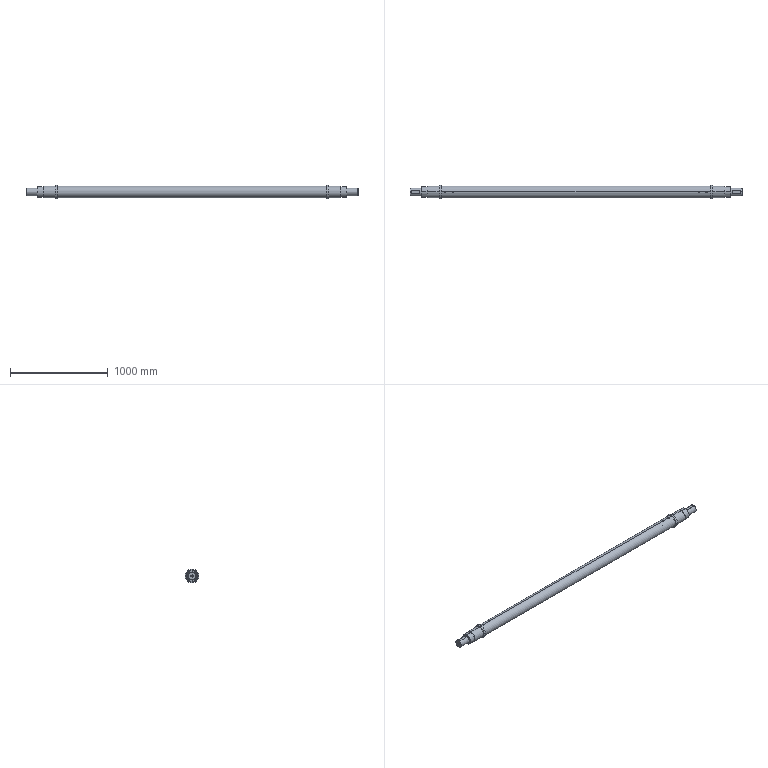Part | STEP file | Drive shaft | 3 solids | 108 faces | box 3402 x 140 x 140 mm | volume 19524168 mm3 | cylinder 54 | plane 22 | cone 20 | torus 12 | commonest cylinder face diameters 16 x16 101 x8 24 x6 21 x4 80 x4 110 x4